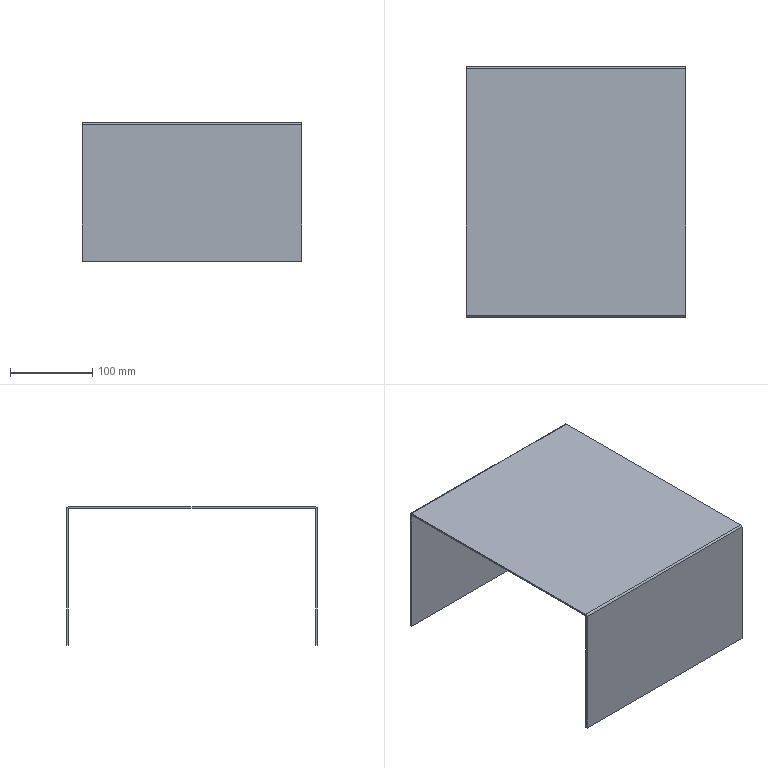Part | STEP file | Oil Filler Tank | 1 solid | 14 faces | box 267 x 305 x 168.5 mm | volume 340188 mm3 | plane 10 | cylinder 4 | commonest cylinder face diameters 0.2 x2 4.2 x2
STEP:
#1=CARTESIAN_POINT('',(-59.5,-990.643,0.));
#2=VERTEX_POINT('',#1);
#3=CARTESIAN_POINT('',(-59.5,-689.843,0.));
#4=VERTEX_POINT('',#3);
#5=CARTESIAN_POINT('',(-59.5,0.,0.));
#6=DIRECTION('',(0.,1.,0.));
#7=VECTOR('',#6,1000.);
#8=LINE('',#5,#7);
#9=EDGE_CURVE('',#2,#4,#8,.T.);
#10=ORIENTED_EDGE('',*,*,#9,.T.);
#11=CARTESIAN_POINT('',(-326.5,-689.843,0.));
#12=VERTEX_POINT('',#11);
#13=CARTESIAN_POINT('',(0.,-689.843,0.));
#14=DIRECTION('',(-1.,0.,0.));
#15=VECTOR('',#14,1000.);
#16=LINE('',#13,#15);
#17=EDGE_CURVE('',#4,#12,#16,.T.);
#18=ORIENTED_EDGE('',*,*,#17,.T.);
#19=CARTESIAN_POINT('',(-326.5,-990.643,0.));
#20=VERTEX_POINT('',#19);
#21=CARTESIAN_POINT('',(-326.5,0.,0.));
#22=DIRECTION('',(0.,-1.,0.));
#23=VECTOR('',#22,1000.);
#24=LINE('',#21,#23);
#25=EDGE_CURVE('',#12,#20,#24,.T.);
#26=ORIENTED_EDGE('',*,*,#25,.T.);
#27=CARTESIAN_POINT('',(0.,-990.643,0.));
#28=DIRECTION('',(1.,0.,0.));
#29=VECTOR('',#28,1000.);
#30=LINE('',#27,#29);
#31=EDGE_CURVE('',#20,#2,#30,.T.);
#32=ORIENTED_EDGE('',*,*,#31,.T.);
#33=EDGE_LOOP('',(#10,#18,#26,#32));
#34=FACE_OUTER_BOUND('',#33,.T.);
#35=CARTESIAN_POINT('',(0.,0.,0.));
#36=DIRECTION('',(0.,0.,1.));
#37=DIRECTION('',(1.,0.,0.));
#38=AXIS2_PLACEMENT_3D('',#35,#36,#37);
#39=PLANE('',#38);
#40=ADVANCED_FACE('',(#34),#39,.T.);
#41=CARTESIAN_POINT('',(-59.5,-687.743,-2.1));
#42=VERTEX_POINT('',#41);
#43=CARTESIAN_POINT('',(-326.5,-687.743,-2.1));
#44=VERTEX_POINT('',#43);
#45=CARTESIAN_POINT('',(-59.5,-687.743,-2.1));
#46=DIRECTION('',(-1.,0.,0.));
#47=VECTOR('',#46,1000.);
#48=LINE('',#45,#47);
#49=EDGE_CURVE('',#42,#44,#48,.T.);
#50=ORIENTED_EDGE('',*,*,#49,.T.);
#51=CARTESIAN_POINT('',(-326.5,-689.843,-2.1));
#52=DIRECTION('',(1.,0.,0.));
#53=DIRECTION('',(0.,0.,-1.));
#54=AXIS2_PLACEMENT_3D('',#51,#52,#53);
#55=CIRCLE('',#54,2.1);
#56=EDGE_CURVE('',#44,#12,#55,.T.);
#57=ORIENTED_EDGE('',*,*,#56,.T.);
#58=ORIENTED_EDGE('',*,*,#17,.F.);
#59=CARTESIAN_POINT('',(-59.5,-689.843,-2.1));
#60=DIRECTION('',(-1.,0.,0.));
#61=DIRECTION('',(0.,0.,-1.));
#62=AXIS2_PLACEMENT_3D('',#59,#60,#61);
#63=CIRCLE('',#62,2.1);
#64=EDGE_CURVE('',#4,#42,#63,.T.);
#65=ORIENTED_EDGE('',*,*,#64,.T.);
#66=EDGE_LOOP('',(#50,#57,#58,#65));
#67=FACE_OUTER_BOUND('',#66,.T.);
#68=CARTESIAN_POINT('',(-59.5,-689.843,-2.1));
#69=DIRECTION('',(1.,0.,0.));
#70=DIRECTION('',(0.,0.,-1.));
#71=AXIS2_PLACEMENT_3D('',#68,#69,#70);
#72=CYLINDRICAL_SURFACE('',#71,2.1);
#73=ADVANCED_FACE('',(#67),#72,.T.);
#74=CARTESIAN_POINT('',(-59.5,-990.643,-2.));
#75=VERTEX_POINT('',#74);
#76=CARTESIAN_POINT('',(-59.5,-689.843,-2.));
#77=VERTEX_POINT('',#76);
#78=CARTESIAN_POINT('',(-59.5,-992.743,-2.));
#79=DIRECTION('',(0.,1.,0.));
#80=VECTOR('',#79,1000.);
#81=LINE('',#78,#80);
#82=EDGE_CURVE('',#75,#77,#81,.T.);
#83=ORIENTED_EDGE('',*,*,#82,.T.);
#84=CARTESIAN_POINT('',(-59.5,-689.743,-2.1));
#85=VERTEX_POINT('',#84);
#86=CARTESIAN_POINT('',(-59.5,-689.843,-2.1));
#87=DIRECTION('',(-1.,0.,0.));
#88=DIRECTION('',(0.,0.,-1.));
#89=AXIS2_PLACEMENT_3D('',#86,#87,#88);
#90=CIRCLE('',#89,0.1);
#91=EDGE_CURVE('',#77,#85,#90,.T.);
#92=ORIENTED_EDGE('',*,*,#91,.T.);
#93=CARTESIAN_POINT('',(-59.5,-689.743,-168.5));
#94=VERTEX_POINT('',#93);
#95=CARTESIAN_POINT('',(-59.5,-689.743,-168.5));
#96=DIRECTION('',(0.,0.,1.));
#97=VECTOR('',#96,1000.);
#98=LINE('',#95,#97);
#99=EDGE_CURVE('',#94,#85,#98,.T.);
#100=ORIENTED_EDGE('',*,*,#99,.F.);
#101=CARTESIAN_POINT('',(-59.5,-687.743,-168.5));
#102=VERTEX_POINT('',#101);
#103=CARTESIAN_POINT('',(-59.5,-687.743,-168.5));
#104=DIRECTION('',(0.,-1.,0.));
#105=VECTOR('',#104,1000.);
#106=LINE('',#103,#105);
#107=EDGE_CURVE('',#102,#94,#106,.T.);
#108=ORIENTED_EDGE('',*,*,#107,.F.);
#109=CARTESIAN_POINT('',(-59.5,-687.743,0.));
#110=DIRECTION('',(0.,0.,1.));
#111=VECTOR('',#110,1000.);
#112=LINE('',#109,#111);
#113=EDGE_CURVE('',#102,#42,#112,.T.);
#114=ORIENTED_EDGE('',*,*,#113,.T.);
#115=ORIENTED_EDGE('',*,*,#64,.F.);
#116=ORIENTED_EDGE('',*,*,#9,.F.);
#117=CARTESIAN_POINT('',(-59.5,-992.743,-2.1));
#118=VERTEX_POINT('',#117);
#119=CARTESIAN_POINT('',(-59.5,-990.643,-2.1));
#120=DIRECTION('',(-1.,0.,0.));
#121=DIRECTION('',(0.,0.,1.));
#122=AXIS2_PLACEMENT_3D('',#119,#120,#121);
#123=CIRCLE('',#122,2.1);
#124=EDGE_CURVE('',#118,#2,#123,.T.);
#125=ORIENTED_EDGE('',*,*,#124,.F.);
#126=CARTESIAN_POINT('',(-59.5,-992.743,-168.5));
#127=VERTEX_POINT('',#126);
#128=CARTESIAN_POINT('',(-59.5,-992.743,0.));
#129=DIRECTION('',(0.,0.,-1.));
#130=VECTOR('',#129,1000.);
#131=LINE('',#128,#130);
#132=EDGE_CURVE('',#118,#127,#131,.T.);
#133=ORIENTED_EDGE('',*,*,#132,.T.);
#134=CARTESIAN_POINT('',(-59.5,-990.743,-168.5));
#135=VERTEX_POINT('',#134);
#136=CARTESIAN_POINT('',(-59.5,-992.743,-168.5));
#137=DIRECTION('',(0.,-1.,0.));
#138=VECTOR('',#137,1000.);
#139=LINE('',#136,#138);
#140=EDGE_CURVE('',#135,#127,#139,.T.);
#141=ORIENTED_EDGE('',*,*,#140,.F.);
#142=CARTESIAN_POINT('',(-59.5,-990.743,-2.1));
#143=VERTEX_POINT('',#142);
#144=CARTESIAN_POINT('',(-59.5,-990.743,-2.));
#145=DIRECTION('',(0.,0.,-1.));
#146=VECTOR('',#145,1000.);
#147=LINE('',#144,#146);
#148=EDGE_CURVE('',#143,#135,#147,.T.);
#149=ORIENTED_EDGE('',*,*,#148,.F.);
#150=CARTESIAN_POINT('',(-59.5,-990.643,-2.1));
#151=DIRECTION('',(-1.,0.,0.));
#152=DIRECTION('',(0.,0.,1.));
#153=AXIS2_PLACEMENT_3D('',#150,#151,#152);
#154=CIRCLE('',#153,0.1);
#155=EDGE_CURVE('',#143,#75,#154,.T.);
#156=ORIENTED_EDGE('',*,*,#155,.T.);
#157=EDGE_LOOP('',(#83,#92,#100,#108,#114,#115,#116,#125,#133,#141,#149,#156));
#158=FACE_OUTER_BOUND('',#157,.T.);
#159=CARTESIAN_POINT('',(-59.5,-992.743,-2.));
#160=DIRECTION('',(1.,0.,0.));
#161=DIRECTION('',(0.,0.,-1.));
#162=AXIS2_PLACEMENT_3D('',#159,#160,#161);
#163=PLANE('',#162);
#164=ADVANCED_FACE('',(#158),#163,.T.);
#165=CARTESIAN_POINT('',(-326.5,-992.743,-2.1));
#166=VERTEX_POINT('',#165);
#167=CARTESIAN_POINT('',(-326.5,-992.743,-2.1));
#168=DIRECTION('',(1.,0.,0.));
#169=VECTOR('',#168,1000.);
#170=LINE('',#167,#169);
#171=EDGE_CURVE('',#166,#118,#170,.T.);
#172=ORIENTED_EDGE('',*,*,#171,.T.);
#173=ORIENTED_EDGE('',*,*,#124,.T.);
#174=ORIENTED_EDGE('',*,*,#31,.F.);
#175=CARTESIAN_POINT('',(-326.5,-990.643,-2.1));
#176=DIRECTION('',(1.,0.,0.));
#177=DIRECTION('',(0.,0.,1.));
#178=AXIS2_PLACEMENT_3D('',#175,#176,#177);
#179=CIRCLE('',#178,2.1);
#180=EDGE_CURVE('',#20,#166,#179,.T.);
#181=ORIENTED_EDGE('',*,*,#180,.T.);
#182=EDGE_LOOP('',(#172,#173,#174,#181));
#183=FACE_OUTER_BOUND('',#182,.T.);
#184=CARTESIAN_POINT('',(-326.5,-990.643,-2.1));
#185=DIRECTION('',(-1.,0.,0.));
#186=DIRECTION('',(0.,0.,1.));
#187=AXIS2_PLACEMENT_3D('',#184,#185,#186);
#188=CYLINDRICAL_SURFACE('',#187,2.1);
#189=ADVANCED_FACE('',(#183),#188,.T.);
#190=ORIENTED_EDGE('',*,*,#25,.F.);
#191=ORIENTED_EDGE('',*,*,#56,.F.);
#192=CARTESIAN_POINT('',(-326.5,-687.743,-168.5));
#193=VERTEX_POINT('',#192);
#194=CARTESIAN_POINT('',(-326.5,-687.743,0.));
#195=DIRECTION('',(0.,0.,-1.));
#196=VECTOR('',#195,1000.);
#197=LINE('',#194,#196);
#198=EDGE_CURVE('',#44,#193,#197,.T.);
#199=ORIENTED_EDGE('',*,*,#198,.T.);
#200=CARTESIAN_POINT('',(-326.5,-689.743,-168.5));
#201=VERTEX_POINT('',#200);
#202=CARTESIAN_POINT('',(-326.5,-687.743,-168.5));
#203=DIRECTION('',(0.,1.,0.));
#204=VECTOR('',#203,1000.);
#205=LINE('',#202,#204);
#206=EDGE_CURVE('',#201,#193,#205,.T.);
#207=ORIENTED_EDGE('',*,*,#206,.F.);
#208=CARTESIAN_POINT('',(-326.5,-689.743,-2.1));
#209=VERTEX_POINT('',#208);
#210=CARTESIAN_POINT('',(-326.5,-689.743,-2.));
#211=DIRECTION('',(0.,0.,-1.));
#212=VECTOR('',#211,1000.);
#213=LINE('',#210,#212);
#214=EDGE_CURVE('',#209,#201,#213,.T.);
#215=ORIENTED_EDGE('',*,*,#214,.F.);
#216=CARTESIAN_POINT('',(-326.5,-689.843,-2.));
#217=VERTEX_POINT('',#216);
#218=CARTESIAN_POINT('',(-326.5,-689.843,-2.1));
#219=DIRECTION('',(1.,0.,0.));
#220=DIRECTION('',(0.,0.,-1.));
#221=AXIS2_PLACEMENT_3D('',#218,#219,#220);
#222=CIRCLE('',#221,0.1);
#223=EDGE_CURVE('',#209,#217,#222,.T.);
#224=ORIENTED_EDGE('',*,*,#223,.T.);
#225=CARTESIAN_POINT('',(-326.5,-990.643,-2.));
#226=VERTEX_POINT('',#225);
#227=CARTESIAN_POINT('',(-326.5,-687.743,-2.));
#228=DIRECTION('',(0.,-1.,0.));
#229=VECTOR('',#228,1000.);
#230=LINE('',#227,#229);
#231=EDGE_CURVE('',#217,#226,#230,.T.);
#232=ORIENTED_EDGE('',*,*,#231,.T.);
#233=CARTESIAN_POINT('',(-326.5,-990.743,-2.1));
#234=VERTEX_POINT('',#233);
#235=CARTESIAN_POINT('',(-326.5,-990.643,-2.1));
#236=DIRECTION('',(-1.,0.,0.));
#237=DIRECTION('',(0.,0.,1.));
#238=AXIS2_PLACEMENT_3D('',#235,#236,#237);
#239=CIRCLE('',#238,0.1);
#240=EDGE_CURVE('',#234,#226,#239,.T.);
#241=ORIENTED_EDGE('',*,*,#240,.F.);
#242=CARTESIAN_POINT('',(-326.5,-990.743,-168.5));
#243=VERTEX_POINT('',#242);
#244=CARTESIAN_POINT('',(-326.5,-990.743,-168.5));
#245=DIRECTION('',(0.,0.,1.));
#246=VECTOR('',#245,1000.);
#247=LINE('',#244,#246);
#248=EDGE_CURVE('',#243,#234,#247,.T.);
#249=ORIENTED_EDGE('',*,*,#248,.F.);
#250=CARTESIAN_POINT('',(-326.5,-992.743,-168.5));
#251=VERTEX_POINT('',#250);
#252=CARTESIAN_POINT('',(-326.5,-992.743,-168.5));
#253=DIRECTION('',(0.,1.,0.));
#254=VECTOR('',#253,1000.);
#255=LINE('',#252,#254);
#256=EDGE_CURVE('',#251,#243,#255,.T.);
#257=ORIENTED_EDGE('',*,*,#256,.F.);
#258=CARTESIAN_POINT('',(-326.5,-992.743,0.));
#259=DIRECTION('',(0.,0.,1.));
#260=VECTOR('',#259,1000.);
#261=LINE('',#258,#260);
#262=EDGE_CURVE('',#251,#166,#261,.T.);
#263=ORIENTED_EDGE('',*,*,#262,.T.);
#264=ORIENTED_EDGE('',*,*,#180,.F.);
#265=EDGE_LOOP('',(#190,#191,#199,#207,#215,#224,#232,#241,#249,#257,#263,#264));
#266=FACE_OUTER_BOUND('',#265,.T.);
#267=CARTESIAN_POINT('',(-326.5,-687.743,-2.));
#268=DIRECTION('',(-1.,0.,0.));
#269=DIRECTION('',(0.,-1.,0.));
#270=AXIS2_PLACEMENT_3D('',#267,#268,#269);
#271=PLANE('',#270);
#272=ADVANCED_FACE('',(#266),#271,.T.);
#273=ORIENTED_EDGE('',*,*,#113,.F.);
#274=CARTESIAN_POINT('',(0.,-687.743,-168.5));
#275=DIRECTION('',(1.,0.,0.));
#276=VECTOR('',#275,1000.);
#277=LINE('',#274,#276);
#278=EDGE_CURVE('',#193,#102,#277,.T.);
#279=ORIENTED_EDGE('',*,*,#278,.F.);
#280=ORIENTED_EDGE('',*,*,#198,.F.);
#281=ORIENTED_EDGE('',*,*,#49,.F.);
#282=EDGE_LOOP('',(#273,#279,#280,#281));
#283=FACE_OUTER_BOUND('',#282,.T.);
#284=CARTESIAN_POINT('',(0.,-687.743,0.));
#285=DIRECTION('',(0.,-1.,0.));
#286=DIRECTION('',(0.,0.,-1.));
#287=AXIS2_PLACEMENT_3D('',#284,#285,#286);
#288=PLANE('',#287);
#289=ADVANCED_FACE('',(#283),#288,.F.);
#290=ORIENTED_EDGE('',*,*,#231,.F.);
#291=CARTESIAN_POINT('',(0.,-689.843,-2.));
#292=DIRECTION('',(-1.,0.,0.));
#293=VECTOR('',#292,1000.);
#294=LINE('',#291,#293);
#295=EDGE_CURVE('',#77,#217,#294,.T.);
#296=ORIENTED_EDGE('',*,*,#295,.F.);
#297=ORIENTED_EDGE('',*,*,#82,.F.);
#298=CARTESIAN_POINT('',(0.,-990.643,-2.));
#299=DIRECTION('',(1.,0.,0.));
#300=VECTOR('',#299,1000.);
#301=LINE('',#298,#300);
#302=EDGE_CURVE('',#226,#75,#301,.T.);
#303=ORIENTED_EDGE('',*,*,#302,.F.);
#304=EDGE_LOOP('',(#290,#296,#297,#303));
#305=FACE_OUTER_BOUND('',#304,.T.);
#306=CARTESIAN_POINT('',(0.,0.,-2.));
#307=DIRECTION('',(0.,0.,1.));
#308=DIRECTION('',(1.,0.,0.));
#309=AXIS2_PLACEMENT_3D('',#306,#307,#308);
#310=PLANE('',#309);
#311=ADVANCED_FACE('',(#305),#310,.F.);
#312=ORIENTED_EDGE('',*,*,#262,.F.);
#313=CARTESIAN_POINT('',(0.,-992.743,-168.5));
#314=DIRECTION('',(-1.,0.,0.));
#315=VECTOR('',#314,1000.);
#316=LINE('',#313,#315);
#317=EDGE_CURVE('',#127,#251,#316,.T.);
#318=ORIENTED_EDGE('',*,*,#317,.F.);
#319=ORIENTED_EDGE('',*,*,#132,.F.);
#320=ORIENTED_EDGE('',*,*,#171,.F.);
#321=EDGE_LOOP('',(#312,#318,#319,#320));
#322=FACE_OUTER_BOUND('',#321,.T.);
#323=CARTESIAN_POINT('',(0.,-992.743,0.));
#324=DIRECTION('',(0.,1.,0.));
#325=DIRECTION('',(0.,0.,1.));
#326=AXIS2_PLACEMENT_3D('',#323,#324,#325);
#327=PLANE('',#326);
#328=ADVANCED_FACE('',(#322),#327,.F.);
#329=ORIENTED_EDGE('',*,*,#206,.T.);
#330=ORIENTED_EDGE('',*,*,#278,.T.);
#331=ORIENTED_EDGE('',*,*,#107,.T.);
#332=CARTESIAN_POINT('',(-326.5,-689.743,-168.5));
#333=DIRECTION('',(1.,0.,0.));
#334=VECTOR('',#333,1000.);
#335=LINE('',#332,#334);
#336=EDGE_CURVE('',#201,#94,#335,.T.);
#337=ORIENTED_EDGE('',*,*,#336,.F.);
#338=EDGE_LOOP('',(#329,#330,#331,#337));
#339=FACE_OUTER_BOUND('',#338,.T.);
#340=CARTESIAN_POINT('',(-326.5,-687.743,-168.5));
#341=DIRECTION('',(0.,0.,1.));
#342=DIRECTION('',(0.,-1.,0.));
#343=AXIS2_PLACEMENT_3D('',#340,#341,#342);
#344=PLANE('',#343);
#345=ADVANCED_FACE('',(#339),#344,.F.);
#346=ORIENTED_EDGE('',*,*,#155,.F.);
#347=CARTESIAN_POINT('',(-326.5,-990.743,-2.1));
#348=DIRECTION('',(1.,0.,0.));
#349=VECTOR('',#348,1000.);
#350=LINE('',#347,#349);
#351=EDGE_CURVE('',#234,#143,#350,.T.);
#352=ORIENTED_EDGE('',*,*,#351,.F.);
#353=ORIENTED_EDGE('',*,*,#240,.T.);
#354=ORIENTED_EDGE('',*,*,#302,.T.);
#355=EDGE_LOOP('',(#346,#352,#353,#354));
#356=FACE_OUTER_BOUND('',#355,.T.);
#357=CARTESIAN_POINT('',(-326.5,-990.643,-2.1));
#358=DIRECTION('',(-1.,0.,0.));
#359=DIRECTION('',(0.,0.,1.));
#360=AXIS2_PLACEMENT_3D('',#357,#358,#359);
#361=CYLINDRICAL_SURFACE('',#360,0.1);
#362=ADVANCED_FACE('',(#356),#361,.F.);
#363=ORIENTED_EDGE('',*,*,#223,.F.);
#364=CARTESIAN_POINT('',(-59.5,-689.743,-2.1));
#365=DIRECTION('',(-1.,0.,0.));
#366=VECTOR('',#365,1000.);
#367=LINE('',#364,#366);
#368=EDGE_CURVE('',#85,#209,#367,.T.);
#369=ORIENTED_EDGE('',*,*,#368,.F.);
#370=ORIENTED_EDGE('',*,*,#91,.F.);
#371=ORIENTED_EDGE('',*,*,#295,.T.);
#372=EDGE_LOOP('',(#363,#369,#370,#371));
#373=FACE_OUTER_BOUND('',#372,.T.);
#374=CARTESIAN_POINT('',(-59.5,-689.843,-2.1));
#375=DIRECTION('',(1.,0.,0.));
#376=DIRECTION('',(0.,0.,-1.));
#377=AXIS2_PLACEMENT_3D('',#374,#375,#376);
#378=CYLINDRICAL_SURFACE('',#377,0.1);
#379=ADVANCED_FACE('',(#373),#378,.F.);
#380=ORIENTED_EDGE('',*,*,#140,.T.);
#381=ORIENTED_EDGE('',*,*,#317,.T.);
#382=ORIENTED_EDGE('',*,*,#256,.T.);
#383=CARTESIAN_POINT('',(-59.5,-990.743,-168.5));
#384=DIRECTION('',(-1.,0.,0.));
#385=VECTOR('',#384,1000.);
#386=LINE('',#383,#385);
#387=EDGE_CURVE('',#135,#243,#386,.T.);
#388=ORIENTED_EDGE('',*,*,#387,.F.);
#389=EDGE_LOOP('',(#380,#381,#382,#388));
#390=FACE_OUTER_BOUND('',#389,.T.);
#391=CARTESIAN_POINT('',(-59.5,-992.743,-168.5));
#392=DIRECTION('',(0.,0.,1.));
#393=DIRECTION('',(0.,-1.,0.));
#394=AXIS2_PLACEMENT_3D('',#391,#392,#393);
#395=PLANE('',#394);
#396=ADVANCED_FACE('',(#390),#395,.F.);
#397=ORIENTED_EDGE('',*,*,#214,.T.);
#398=ORIENTED_EDGE('',*,*,#336,.T.);
#399=ORIENTED_EDGE('',*,*,#99,.T.);
#400=ORIENTED_EDGE('',*,*,#368,.T.);
#401=EDGE_LOOP('',(#397,#398,#399,#400));
#402=FACE_OUTER_BOUND('',#401,.T.);
#403=CARTESIAN_POINT('',(0.,-689.743,0.));
#404=DIRECTION('',(0.,-1.,0.));
#405=DIRECTION('',(0.,0.,-1.));
#406=AXIS2_PLACEMENT_3D('',#403,#404,#405);
#407=PLANE('',#406);
#408=ADVANCED_FACE('',(#402),#407,.T.);
#409=ORIENTED_EDGE('',*,*,#148,.T.);
#410=ORIENTED_EDGE('',*,*,#387,.T.);
#411=ORIENTED_EDGE('',*,*,#248,.T.);
#412=ORIENTED_EDGE('',*,*,#351,.T.);
#413=EDGE_LOOP('',(#409,#410,#411,#412));
#414=FACE_OUTER_BOUND('',#413,.T.);
#415=CARTESIAN_POINT('',(0.,-990.743,0.));
#416=DIRECTION('',(0.,1.,0.));
#417=DIRECTION('',(0.,0.,1.));
#418=AXIS2_PLACEMENT_3D('',#415,#416,#417);
#419=PLANE('',#418);
#420=ADVANCED_FACE('',(#414),#419,.T.);
#421=CLOSED_SHELL('',(#40,#73,#164,#189,#272,#289,#311,#328,#345,#362,#379,#396,#408,#420));
#422=MANIFOLD_SOLID_BREP('',#421);
#423=CARTESIAN_POINT('',(0.,0.,0.));
#424=DIRECTION('',(0.,0.,1.));
#425=DIRECTION('',(1.,0.,0.));
#426=AXIS2_PLACEMENT_3D('',#423,#424,#425);
#427=(LENGTH_UNIT()NAMED_UNIT(*)SI_UNIT(.MILLI.,.METRE.));
#428=UNCERTAINTY_MEASURE_WITH_UNIT(LENGTH_MEASURE(0.00001),#427,'','');
#429=(NAMED_UNIT(*)PLANE_ANGLE_UNIT()SI_UNIT($,.RADIAN.));
#430=(NAMED_UNIT(*)SI_UNIT($,.STERADIAN.)SOLID_ANGLE_UNIT());
#431=(GEOMETRIC_REPRESENTATION_CONTEXT(3)GLOBAL_UNCERTAINTY_ASSIGNED_CONTEXT((#428))GLOBAL_UNIT_ASSIGNED_CONTEXT((#427,#429,#430))REPRESENTATION_CONTEXT('',''));
#432=ADVANCED_BREP_SHAPE_REPRESENTATION('',(#422,#426),#431);